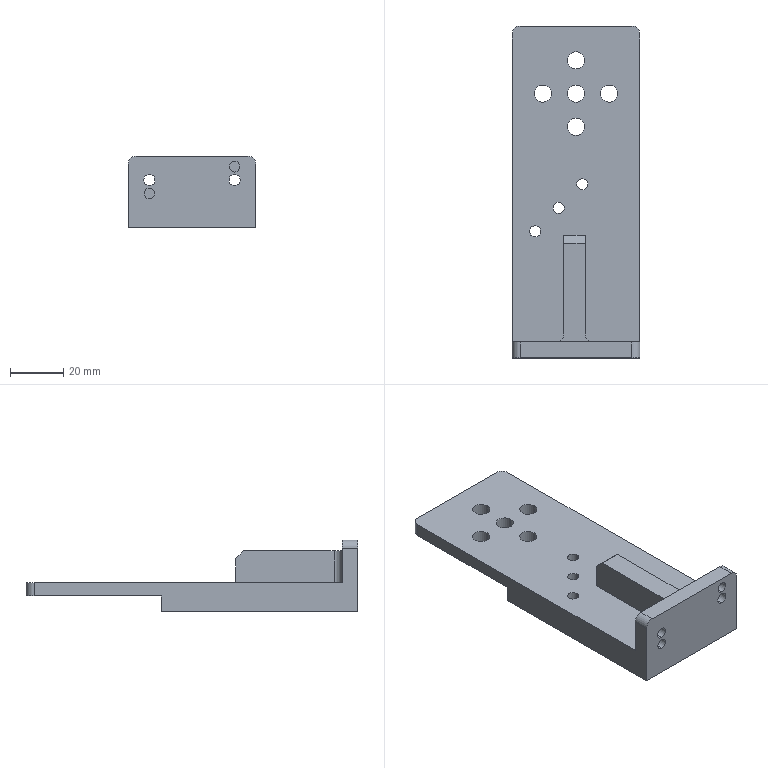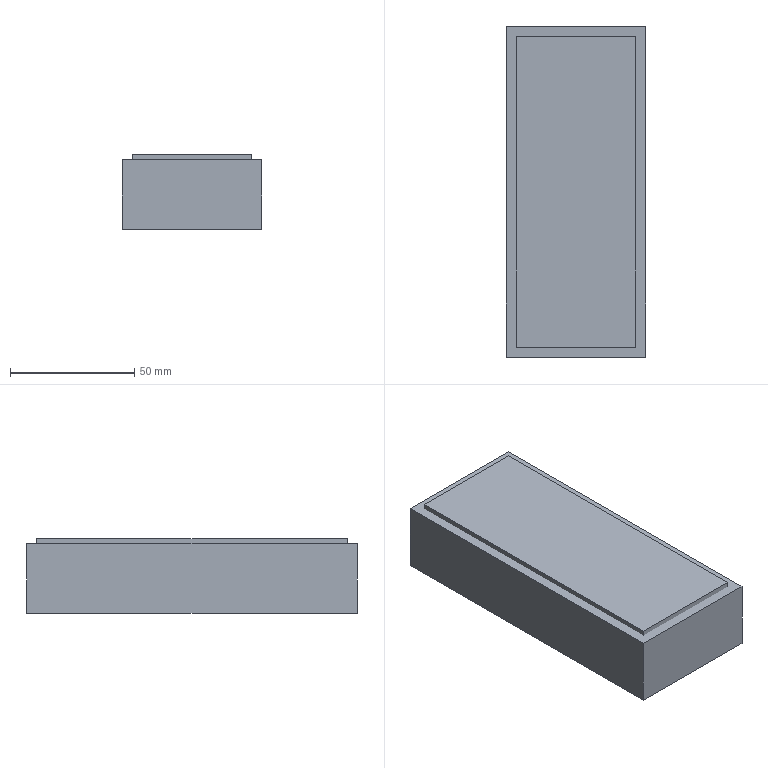CAM job | NX | 3+2 milling, drilling | part box 48 x 124.7 x 27 mm | stock box 56 x 132.7 x 30 mm
Tools:
number,name,description,diameter,corner_radius,flute_length,length,flutes
19,D80,Milling Tool-5 Parameters,80.0,0.0,50.0,75.0,2
15,D10,Milling Tool-5 Parameters,10.0,0.0,50.0,75.0,2
14,D10JING,Milling Tool-5 Parameters,10.0,0.0,50.0,75.0,2
1,D6A45,Milling Tool-5 Parameters,6.0,0.0,50.0,75.0,2
10,6.5ZT,Drilling Tool,6.5,0.0,35.0,50.0,2
16,D6R0.5,Milling Tool-5 Parameters,6.0,0.5,50.0,75.0,2
4,4.2ZT,Drilling Tool,4.2,0.0,35.0,50.0,2
12,D6,Milling Tool-5 Parameters,6.0,0.0,50.0,75.0,2
3,D3,Milling Tool-5 Parameters,3.0,0.0,50.0,75.0,2
Operations:
program,operation,operation_type,tool,method,geometry_group,spindle_rpm,surface_speed,feed_per_tooth,feed_cut,feed_plunge,cut_length_mm,path_length_mm,cut_time_min,machine_time_min
1,FLOOR_WALL_COPY,VolumeBased25DMillingOperation,D80,METHOD,A,6500.0,1633.0,0.1154,1500.0,100.0,228.7,282.7,0.1525,0.1579
1,ADAPTIVE_MILLING,CavityMilling,D10,METHOD,A,9500.0,298.0,0.1579,3000.0,1000.0,6412.159,6731.919,2.143,2.175
1,ADAPTIVE_MILLING_COPY,CavityMilling,D10,METHOD,A,9500.0,298.0,0.1579,3000.0,1000.0,1549.375,1657.375,0.5185,0.5293
1,ZLEVEL_PROFILE_COPY_1_COPY_COPY_1_COPY,ZLevelMilling,D10JING,METHOD,A,9500.0,298.0,0.0632,1200.0,1000.0,763.158,963.518,0.6372,0.6572
1,FLOOR_WALL_1,VolumeBased25DMillingOperation,D10JING,METHOD,A,9500.0,298.0,0.0658,1250.0,100.0,764.373,960.375,0.6115,0.6311
1,DRILLING_COPY_1,Operation,D6A45,METHOD,A,5000.0,94.0,0.035,350.0,0.0,32.0,260.175,0.0914,0.1142
1,DRILLING_COPY_1_COPY_1_1,Operation,6.5ZT,METHOD,A,2000.0,34.0,0.05,200.0,0.0,57.264,260.099,0.2863,0.3066
1,DRILLING_COPY_1_COPY_1_1_COPY,Operation,4.2ZT,METHOD,A,2000.0,34.0,0.05,200.0,0.0,50.285,204.605,0.2514,0.2669
1,PLANAR_MILL_COPY_COPY_COPY_COPY_COPY_COPY_1_COPY_1,PlanarMilling,D6A45,METHOD,A,9500.0,179.0,0.0658,1250.0,100.0,301.456,600.214,0.2412,0.271
1,PLANAR_MILL_COPY_COPY_COPY_COPY_COPY_COPY_1_COPY_1_COPY,PlanarMilling,D6A45,METHOD,A,9500.0,179.0,0.0658,1250.0,100.0,260.363,778.0,0.2083,0.2601
2,FLOOR_WALL_COPY_COPY,VolumeBased25DMillingOperation,D80,METHOD,B,6500.0,1633.0,0.1154,1500.0,100.0,662.1,1247.501,0.4414,0.4999
2,FLOOR_WALL,VolumeBased25DMillingOperation,D10,METHOD,B,9500.0,298.0,0.1579,3000.0,1000.0,12405.287,12615.868,4.155,4.176
2,FLOOR_WALL_COPY_2,VolumeBased25DMillingOperation,D10,METHOD,B,9500.0,298.0,0.1579,3000.0,1000.0,1995.891,2057.691,0.669,0.6752
2,FLOOR_WALL_COPY_1,VolumeBased25DMillingOperation,D10JING,METHOD,B,9500.0,298.0,0.0632,1200.0,1000.0,1640.273,2054.61,1.371,1.413
2,ZLEVEL_PROFILE,ZLevelMilling,D6,METHOD,B,9500.0,179.0,0.0842,1600.0,100.0,352.703,652.354,0.2204,0.2504
2,ZLEVEL_PROFILE_1,ZLevelMilling,D6R0.5,METHOD,B,9500.0,119.0,0.1842,3500.0,100.0,812.393,982.239,0.2321,0.2491
2,ZLEVEL_PROFILE_1_COPY,ZLevelMilling,D6R0.5,METHOD,B,9500.0,119.0,0.1842,3500.0,100.0,457.23,522.739,0.1306,0.1372
2,PLANAR_MILL_COPY_COPY_COPY_COPY_COPY_COPY_1_COPY_1_COPY_1,PlanarMilling,D6A45,METHOD,B,9500.0,179.0,0.0658,1250.0,100.0,442.424,1466.32,0.3539,0.4563
2,PLANAR_MILL_COPY_COPY_COPY_COPY_COPY_COPY_1_COPY_1_COPY_1_COPY,PlanarMilling,D6A45,METHOD,B,9500.0,179.0,0.0658,1250.0,100.0,90.053,157.053,0.072,0.0787
2,PLANAR_MILL_COPY_COPY_COPY_COPY_COPY_COPY_1_COPY_1_COPY_1_COPY_COPY,PlanarMilling,D6A45,METHOD,B,9500.0,179.0,0.0658,1250.0,100.0,119.394,178.394,0.0955,0.1014
3,DRILLING_COPY_1_COPY,Operation,D6A45,METHOD,C,5000.0,94.0,0.035,350.0,0.0,16.0,144.802,0.0457,0.0586
3,DRILLING_COPY_1_COPY_1_1_COPY_1,Operation,4.2ZT,METHOD,C,2000.0,34.0,0.05,200.0,0.0,23.524,142.188,0.1176,0.1295
3,HOLE_MILLING,CylinderMilling,D3,METHOD,C,9500.0,89.0,0.0658,1250.0,100.0,95.782,254.309,0.0766,0.0925
3,PLANAR_MILL_COPY_COPY_COPY_COPY_COPY_COPY_1_COPY_1_COPY_1_1,PlanarMilling,D6A45,METHOD,C,9500.0,179.0,0.0658,1250.0,100.0,62.606,342.72,0.0501,0.0781
3,刀补3,CylinderMilling,D3,METHOD,C,9500.0,89.0,0.0526,1000.0,100.0,29.446,187.972,0.0294,0.0453